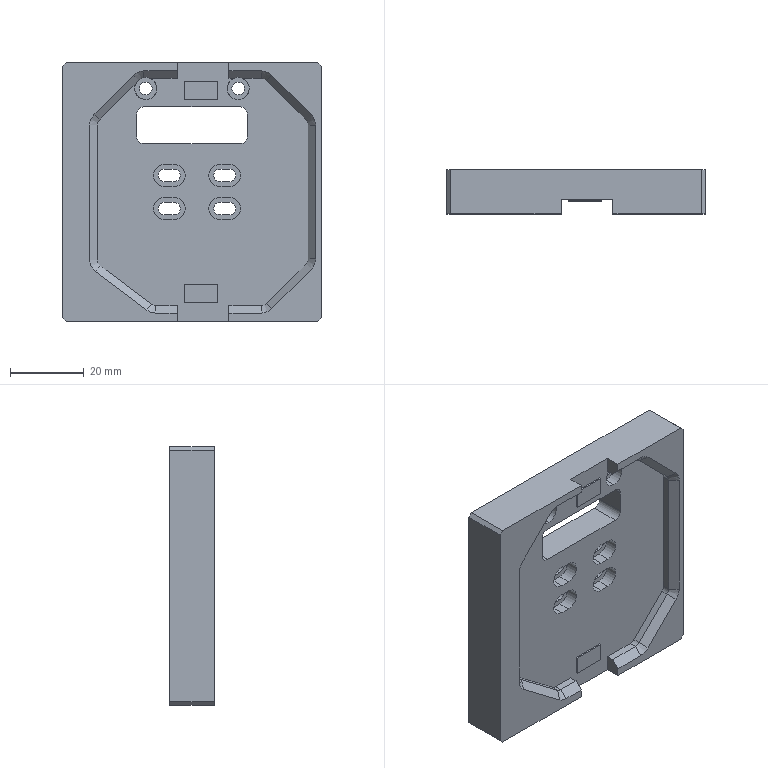Part | STEP file | lift positioning block | 1 solid | 116 faces | box 70 x 12 x 70 mm | volume 41545 mm3 | plane 73 | cylinder 35 | cone 8 | commonest cylinder face diameters 3.4 x12 6 x12 4 x11